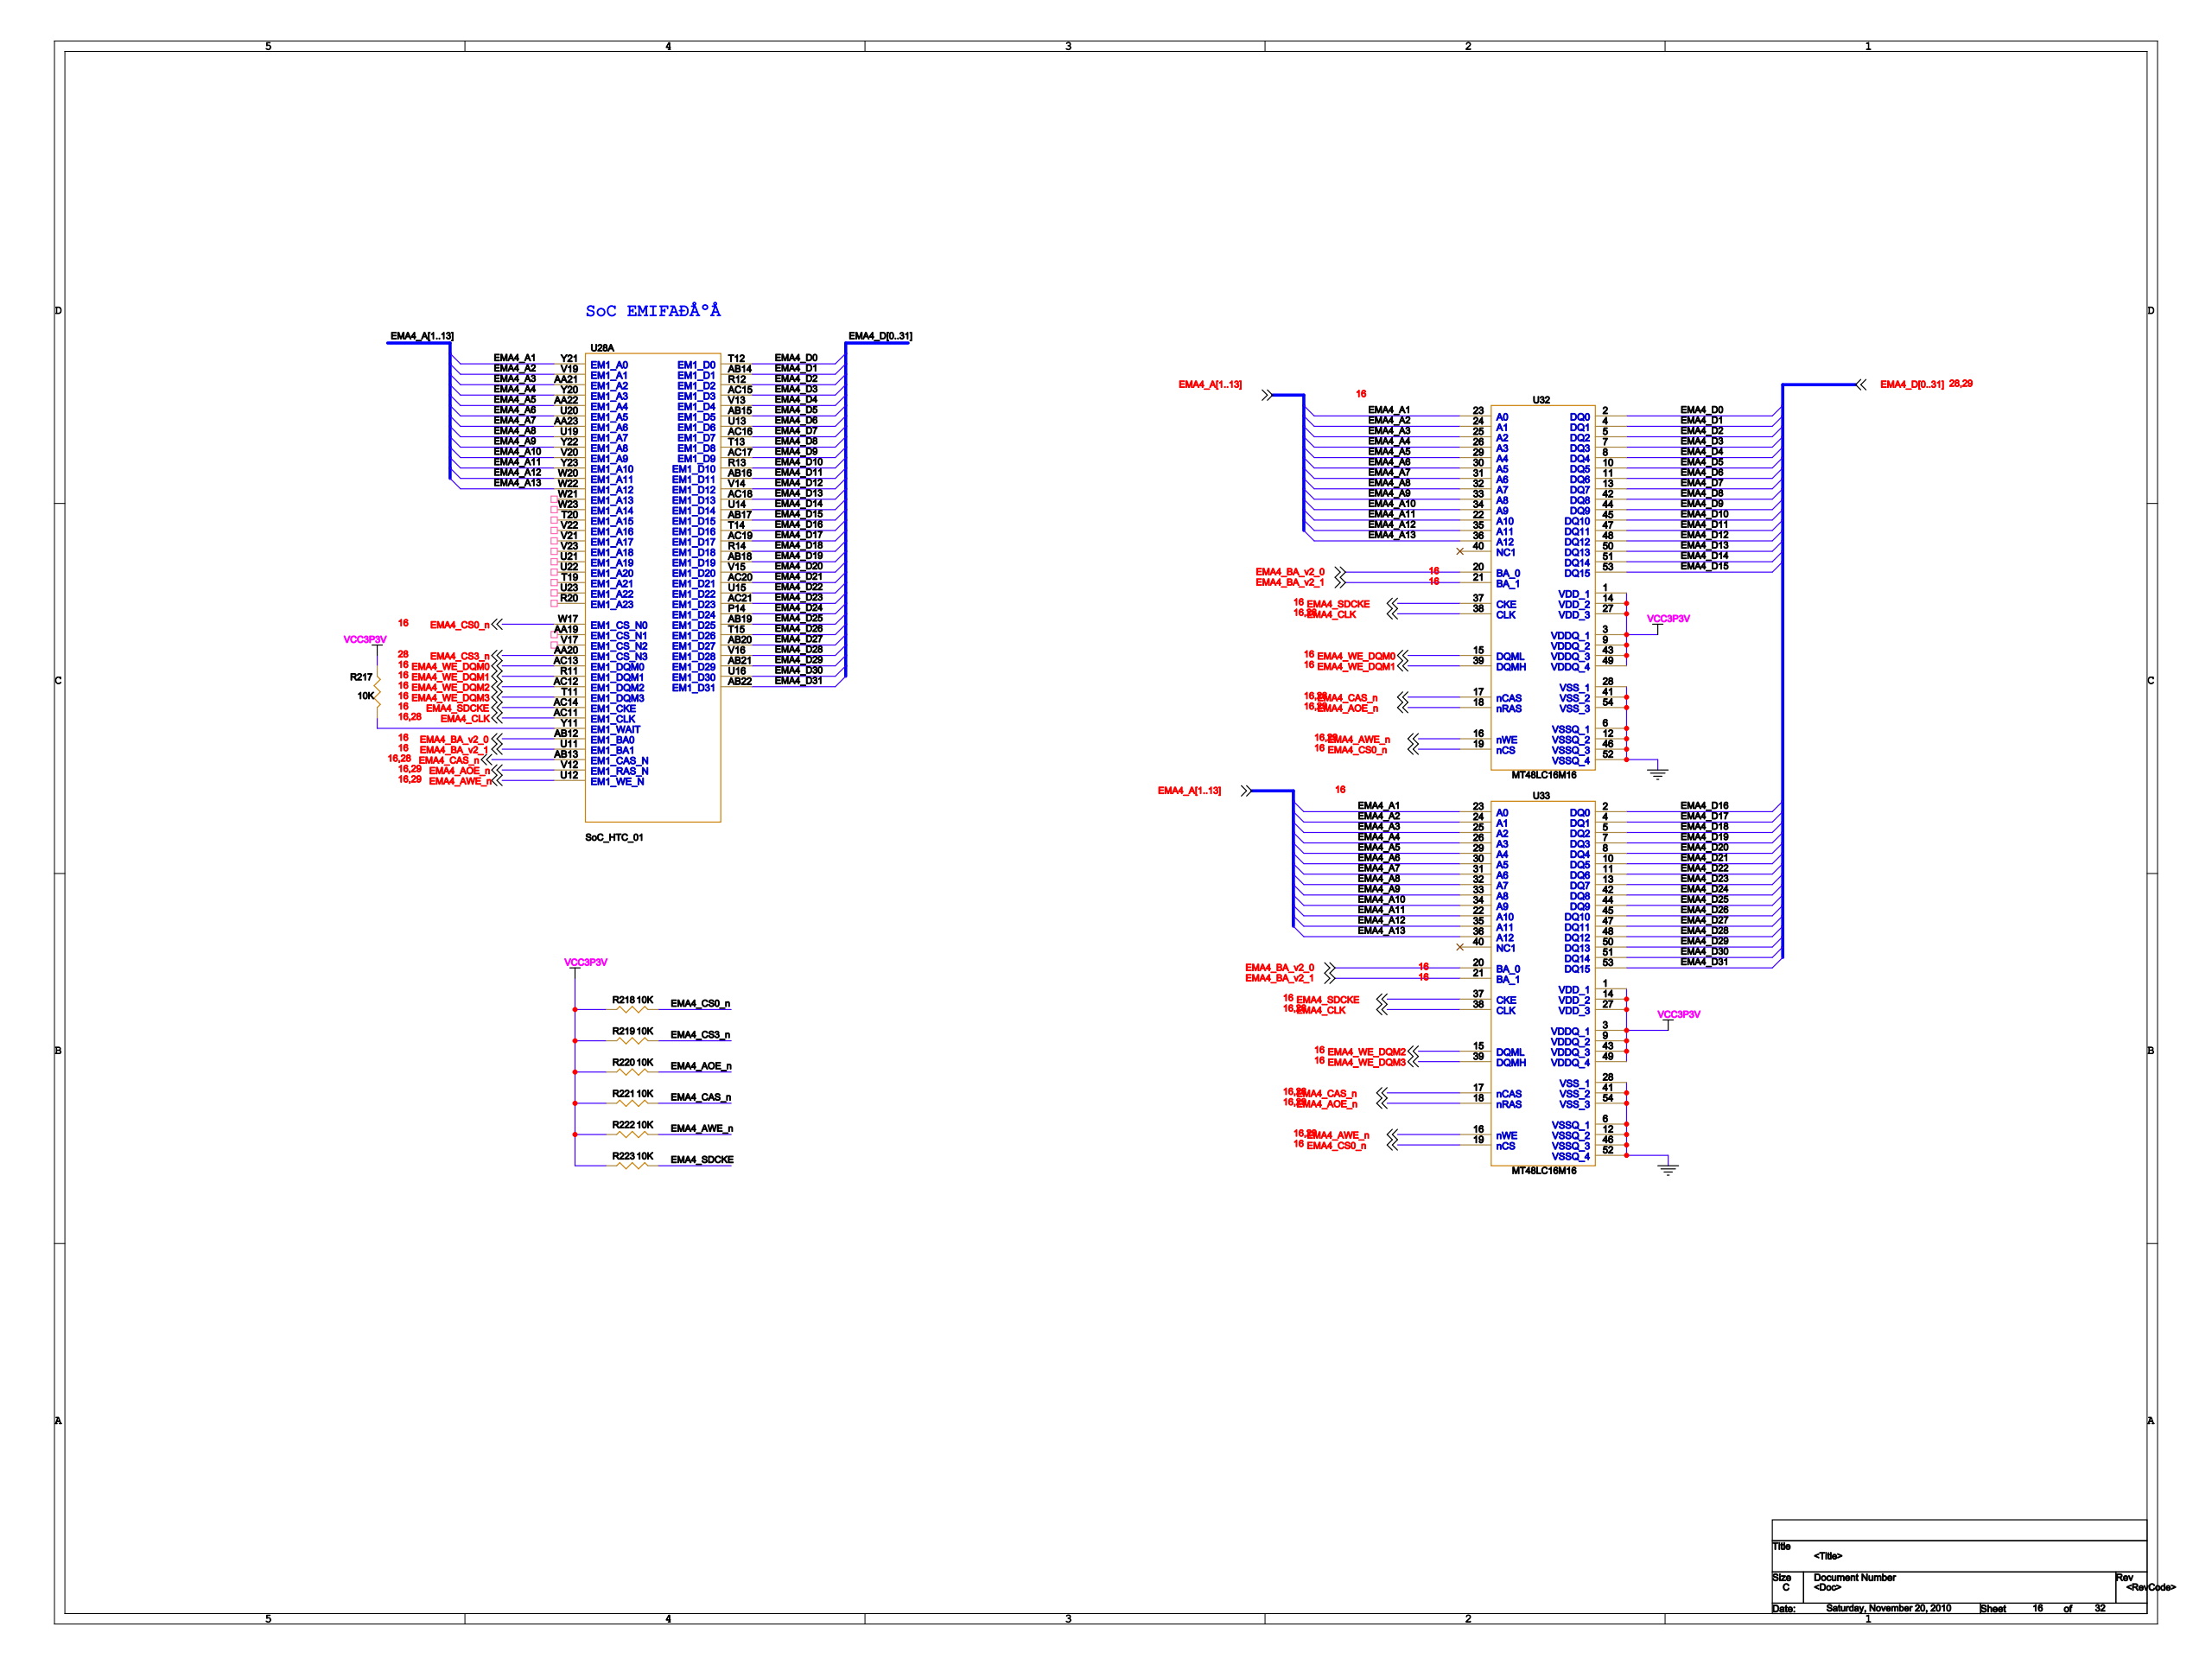Circuit board | Cadence Allegro | 1001 parts | 1318 nets | one sheet of the schematic
Parts on this sheet (reference | value | footprint):
R217 | 10K | 0603
R218 | 10K | 0603
R219 | 10K | 0603
R220 | 10K | 0603
R221 | 10K | 0603
R222 | 10K | 0603
R223 | 10K | 0603
U11 | MT48LC32M16 | TSOP54
U14 | MT48LC16M16 | TSOP54
U15 | MT48LC16M16 | TSOP54
U20 | MT48LC16M16 | TSOP54
U21 | MT48LC16M16 | TSOP54
U23 | MT48LC32M16 | TSOP54
U28 | SoC_HTC_01 | L529_XIN
U32 | MT48LC16M16 | TSOP54
U33 | MT48LC16M16 | TSOP54
Nets of these parts (net: part-pin ...):
EMA4_AOE_N: R220-2 U28-V12 U32-18 U33-18
EMA4_D0: U28-T12 U32-2
EMA4_D10: U28-R13 U32-45
EMA4_D8: U28-T13 U32-42
EMA4_D26: U28-T15 U33-45
EMA4_AWE_N: R222-2 U28-U12 U32-16 U33-16
EMA4_D2: U28-R12 U32-5
EMA4_D18: U28-R14 U33-5
EMA4_D16: U28-T14 U33-2
EMA4_D14: U28-U14 U32-51
EMA4_D22: U28-U15 U33-11
EMA4_D6: U28-U13 U32-11
EMA4_D24: U28-P14 U33-42
EMA4_D20: U28-V15 U33-8
EMA4_D12: U28-V14 U32-48
EMA4_CS3_N: R219-2 U28-AA20
EMA4_D30: U28-U16 U33-51
EMA4_D31: U28-AB22 U33-53
EMA4_D29: U28-AB21 U33-50
EMA4_D23: U28-AC21 U33-13
EMA4_D19: U28-AB18 U33-7
EMA4_D15: U28-AB17 U32-53
EMA4_D28: U28-V16 U33-48
EMA4_D4: U28-V13 U32-8
EMA4_D27: U28-AB20 U33-47
EMA4_D21: U28-AC20 U33-10
EMA4_D17: U28-AC19 U33-4
EMA4_D13: U28-AC18 U32-50
EMA4_CLK: U28-AC11 U32-38 U33-38
EMA4_D25: U28-AB19 U33-44
EMA4_D9: U28-AC17 U32-44
EMA4_D7: U28-AC16 U32-13
EMA4_D3: U28-AC15 U32-7
EMA4_CAS_N: R221-2 U28-AB13 U32-17 U33-17
EMA4_D11: U28-AB16 U32-47
EMA4_D5: U28-AB15 U32-10
EMA4_D1: U28-AB14 U32-4
VCC3P3V: R217-2 R218-1 R219-1 R220-1 R221-1 R222-1 R223-1 U11-1 U11-3 U11-9 U11-14 U11-27 U11-43 U11-49 U14-1 U14-3 U14-9 U14-14 U14-27 U14-43 U14-49 U15-1 U15-3 U15-9 U15-14 U15-27 U15-43 U15-49 U20-1 U20-3 U20-9 U20-14 U20-27 U20-43 U20-49 U21-1 U21-3 U21-9 U21-14 U21-27 U21-43 U21-49 U23-1 U23-3 U23-9 U23-14 U23-27 U23-43 U23-49 U32-1 U32-3 U32-9 U32-14 U32-27 U32-43 U32-49 U33-1 U33-3 U33-9 U33-14 U33-27 U33-43 U33-49
EMA4_A1: U28-Y21 U32-23 U33-23
EMA4_A2: U28-V19 U32-24 U33-24
EMA4_A11: U28-Y23 U32-22 U33-22
EMA4_A12: U28-W20 U32-35 U33-35
EMA4_A13: U28-W22 U32-36 U33-36
EMA4_A3: U28-AA21 U32-25 U33-25
EMA4_A4: U28-Y20 U32-26 U33-26
EMA4_A5: U28-AA22 U32-29 U33-29
EMA4_A6: U28-U20 U32-30 U33-30
EMA4_A7: U28-AA23 U32-31 U33-31
EMA4_A8: U28-U19 U32-32 U33-32
EMA4_A9: U28-Y22 U32-33 U33-33
EMA4_A10: U28-V20 U32-34 U33-34
EMA4_SDCKE: R223-2 U28-AC14 U32-37 U33-37
EMA4_CS0_N: R218-2 U28-W17 U32-19 U33-19
EMA4_WE_DQM0: U28-AC13 U32-15
EMA4_WE_DQM1: U28-R11 U32-39
EMA4_WE_DQM2: U28-AC12 U33-15
EMA4_WE_DQM3: U28-T11 U33-39
N16847264: R217-1 U28-Y11